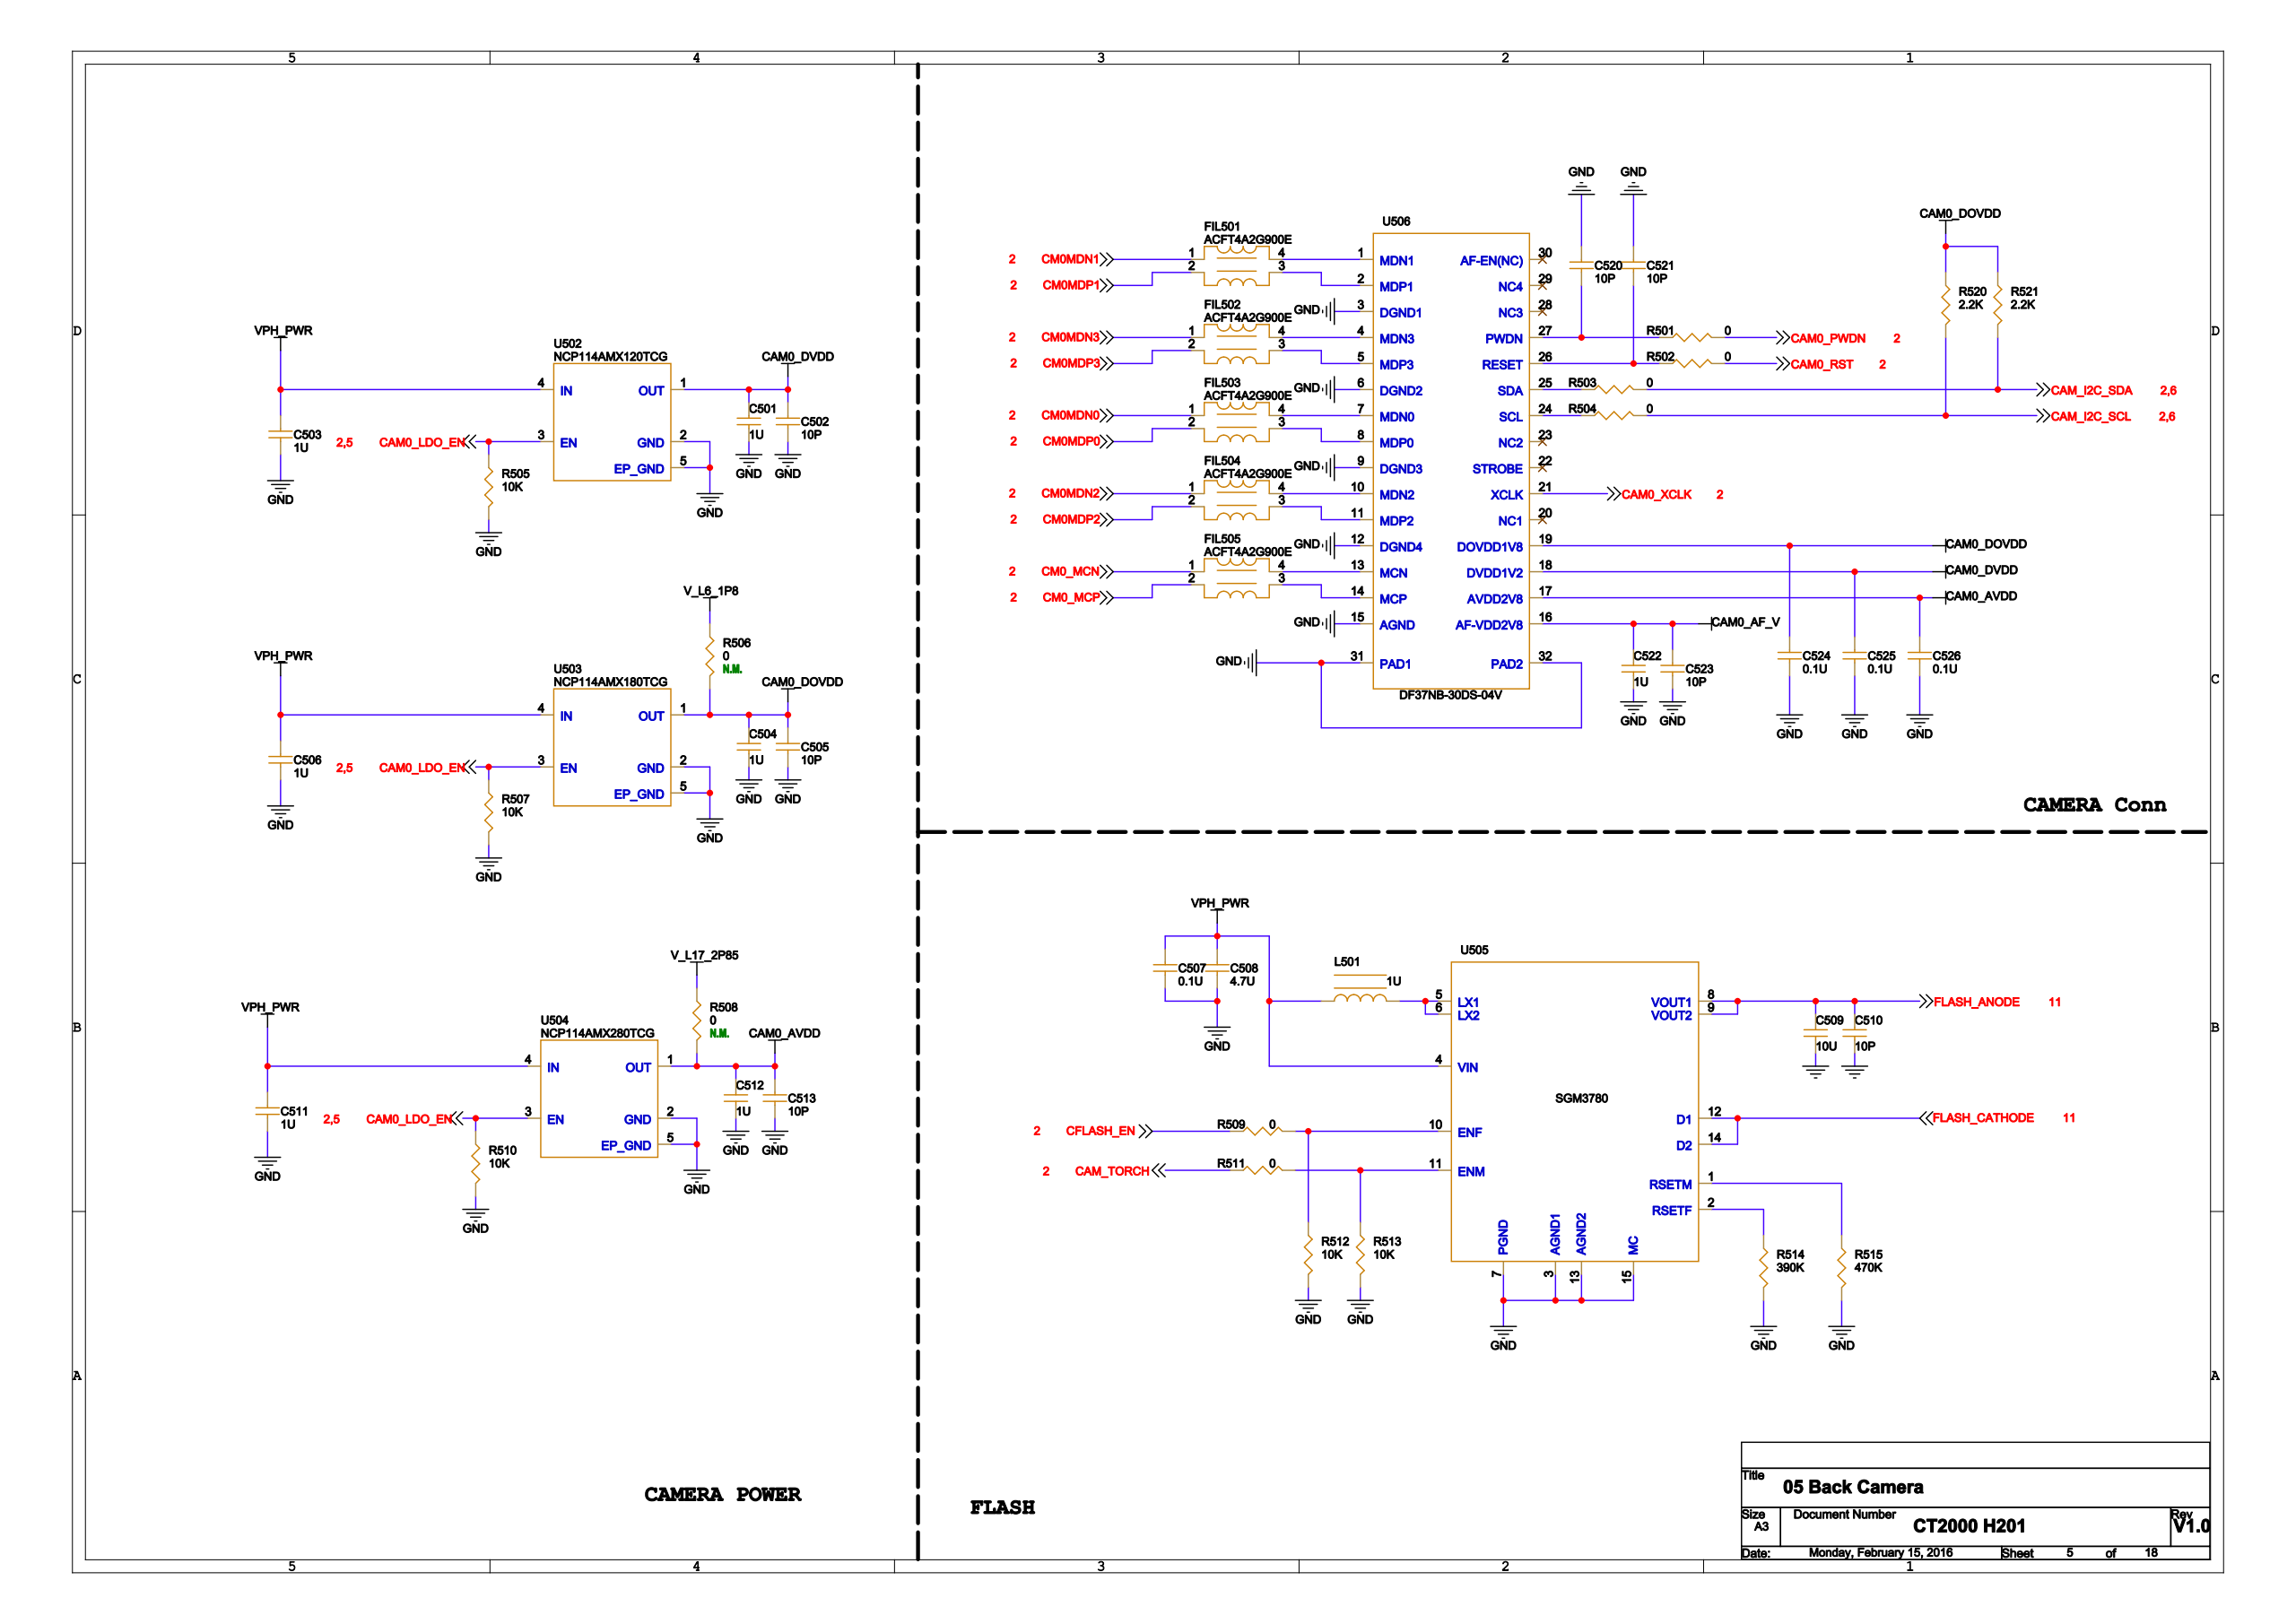Circuit board | Cadence Allegro | 573 parts | 376 nets | one sheet of the schematic
Parts on this sheet (reference | value | footprint):
C501 | 1U | C0402
C502 | 10P | C0402
C503 | 1U | C0402
C504 | 1U | C0402
C505 | 10P | C0402
C506 | 1U | C0402
C507 | 0.1U | C0402
C508 | 4.7U | C0402
C509 | 10U | C0603
C510 | 10P | C0402
C511 | 1U | C0402
C512 | 1U | C0402
C513 | 10P | C0402
C520 | 10P | C0402
C521 | 10P | C0402
C522 | 1U | C0402
C523 | 10P | C0402
C524 | 0.1U | C0402
C525 | 0.1U | C0402
C526 | 0.1U | C0402
FIL501 | ACFT4A2G900E | EMI4_0P85X0P65X0P55_INNOCHIPS
FIL502 | ACFT4A2G900E | EMI4_0P85X0P65X0P55_INNOCHIPS
FIL503 | ACFT4A2G900E | EMI4_0P85X0P65X0P55_INNOCHIPS
FIL504 | ACFT4A2G900E | EMI4_0P85X0P65X0P55_INNOCHIPS
FIL505 | ACFT4A2G900E | EMI4_0P85X0P65X0P55_INNOCHIPS
L501 | 1U | L2520_VLS252010HBX
R501 | 0 | R0402
R502 | 0 | R0402
R503 | 0 | R0402
R504 | 0 | R0402
R505 | 10K | R0402
R506 | 0 | R0402
R507 | 10K | R0402
R508 | 0 | R0402
R509 | 0 | R0402
R510 | 10K | R0402
R511 | 0 | R0402
R512 | 10K | R0402
R513 | 10K | R0402
R514 | 390K | R0402
R515 | 470K | R0402
R520 | 2.2K | R0402
R521 | 2.2K | R0402
U502 | NCP114AMX120TCG | UDFN4_1X1X0P7_0P65
U503 | NCP114AMX180TCG | UDFN4_1X1X0P7_0P65
U504 | NCP114AMX280TCG | UDFN4_1X1X0P7_0P65
U505 | SGM3780 | TDFN14_2X3X0P9_0P4
U506 | DF37NB-30DS-04V | BTB_DF37NB-30DS-04V_CCW
Nets of these parts (net: part-pin ...):
GND: C501-2 C502-2 C503-2 C504-2 C505-2 C506-2 C507-2 C508-2 C509-2 C510-2 C511-2 C512-2 C513-2 C520-1 C521-1 C522-2 C523-2 C524-2 C525-2 C526-2 R505-2 R507-2 R510-2 R512-2 R513-2 R514-2 R515-2 U502-2 U502-5 U503-2 U503-5 U504-2 U504-5 U505-3 U505-7 U505-13 U505-15 U506-3 U506-6 U506-9 U506-12 U506-15 U506-31 U506-32
FLASH_CATHODE: U505-12 U505-14
FLASH_ANODE: C509-1 C510-1 U505-8 U505-9
V_L17_2P85: R508-1
VPH_PWR: C503-1 C506-1 C507-1 C508-1 C511-1 L501-1 U502-4 U503-4 U504-4 U505-4
CAM0_LDO_EN: R505-1 R507-1 R510-1 U502-3 U503-3 U504-3
CAM0_DOVDD: C504-1 C505-1 C524-1 R506-2 R520-1 R521-1 U503-1 U506-19
CAM0_AF_V: C522-1 C523-1 U506-16
CAM0_PWDN: R501-2
CAM0_RST: R502-2
CAM_I2C_SDA: R503-2 R521-2
CAM_I2C_SCL: R504-2 R520-2
CFLASH_EN: R509-1
CM0MDN0: FIL503-1
CM0MDN1: FIL501-1
CM0MDN2: FIL504-1
CM0MDN3: FIL502-1
CM0MDP0: FIL503-2
CM0MDP1: FIL501-2
CM0MDP2: FIL504-2
CM0MDP3: FIL502-2
CM0_MCN: FIL505-1
CM0_MCP: FIL505-2
CAM_TORCH: R511-1
V_L6_1P8: R506-1
CAM0_DVDD: C501-1 C502-1 C525-1 U502-1 U506-18
N51919607: FIL501-3 U506-2
N51919604: FIL501-4 U506-1
N51919668: FIL502-3 U506-5
N51919666: FIL502-4 U506-4
N51919737: FIL503-3 U506-8
N51919735: FIL503-4 U506-7
N51919806: FIL504-3 U506-11
N51919804: FIL504-4 U506-10
N51919875: FIL505-3 U506-14
N51919873: FIL505-4 U506-13
CAM0_AVDD: C512-1 C513-1 C526-1 R508-2 U504-1 U506-17
N51920998: C520-2 R501-1 U506-27
N51921001: C521-2 R502-1 U506-26
N51921007: R504-1 U506-24
N51921004: R503-1 U506-25
CAM0_XCLK: U506-21
N51927784: L501-2 U505-5 U505-6
N51929324: R509-2 R512-1 U505-10
N51929368: R511-2 R513-1 U505-11
N51932627: R514-1 U505-2
N51932766: R515-1 U505-1